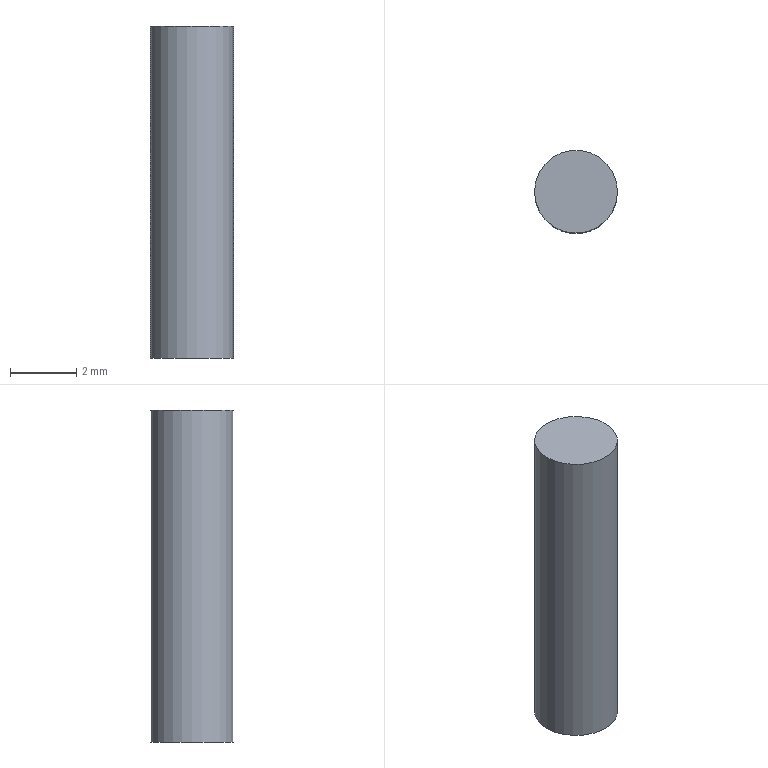Part | STEP file | 1 solid | 3 faces | box 2.5 x 2.5 x 10 mm | volume 49.087 mm3 | plane 2 | cylinder 1 | commonest cylinder face diameters 2.5 x1
STEP:
#1=CARTESIAN_POINT('',(0.,0.,0.));
#2=DIRECTION('',(0.,0.,1.));
#3=DIRECTION('',(1.,0.,0.));
#4=AXIS2_PLACEMENT_3D('',#1,#2,#3);
#5=CARTESIAN_POINT('',(1.25,0.,10.));
#6=VERTEX_POINT('',#5);
#7=CARTESIAN_POINT('',(0.,0.,10.));
#8=DIRECTION('',(0.,0.,-1.));
#9=DIRECTION('',(1.,0.,0.));
#10=AXIS2_PLACEMENT_3D('',#7,#8,#9);
#11=CIRCLE('',#10,1.25);
#12=CARTESIAN_POINT('',(0.,0.,0.));
#13=DIRECTION('',(0.,0.,1.));
#14=DIRECTION('',(1.,0.,0.));
#15=AXIS2_PLACEMENT_3D('',#12,#13,#14);
#16=CYLINDRICAL_SURFACE('',#15,1.25);
#17=CARTESIAN_POINT('',(6.283,10.));
#18=DIRECTION('',(-1.,0.));
#19=VECTOR('',#18,1.);
#20=LINE('',#17,#19);
#21=(GEOMETRIC_REPRESENTATION_CONTEXT(2)PARAMETRIC_REPRESENTATION_CONTEXT()REPRESENTATION_CONTEXT('',''));
#22=DEFINITIONAL_REPRESENTATION('',(#20),#21);
#23=PCURVE('',#16,#22);
#24=CARTESIAN_POINT('',(0.,0.,10.));
#25=DIRECTION('',(0.,0.,1.));
#26=DIRECTION('',(1.,0.,0.));
#27=AXIS2_PLACEMENT_3D('',#24,#25,#26);
#28=PLANE('',#27);
#29=CARTESIAN_POINT('',(1.25,0.));
#30=CARTESIAN_POINT('',(1.25,-2.165));
#31=CARTESIAN_POINT('',(-0.625,-1.083));
#32=CARTESIAN_POINT('',(-2.5,0.));
#33=CARTESIAN_POINT('',(-0.625,1.083));
#34=CARTESIAN_POINT('',(1.25,2.165));
#35=CARTESIAN_POINT('',(1.25,0.));
#36=(BOUNDED_CURVE()B_SPLINE_CURVE(2,(#29,#30,#31,#32,#33,#34,#35),.UNSPECIFIED.,.T.,.F.)B_SPLINE_CURVE_WITH_KNOTS((1,2,2,2,2,1),(-2.094,0.,2.094,4.189,6.283,8.378),.UNSPECIFIED.)CURVE()GEOMETRIC_REPRESENTATION_ITEM()RATIONAL_B_SPLINE_CURVE((1.,0.5,1.,0.5,1.,0.5,1.))REPRESENTATION_ITEM(''));
#37=(GEOMETRIC_REPRESENTATION_CONTEXT(2)PARAMETRIC_REPRESENTATION_CONTEXT()REPRESENTATION_CONTEXT('',''));
#38=DEFINITIONAL_REPRESENTATION('',(#36),#37);
#39=PCURVE('',#28,#38);
#40=SURFACE_CURVE('',#11,(#23,#39),.PCURVE_S1.);
#41=EDGE_CURVE('',#6,#6,#40,.T.);
#42=ORIENTED_EDGE('',*,*,#41,.T.);
#43=CARTESIAN_POINT('',(1.25,0.,0.));
#44=VERTEX_POINT('',#43);
#45=CARTESIAN_POINT('',(1.25,0.,0.));
#46=CARTESIAN_POINT('',(1.25,0.,10.));
#47=B_SPLINE_CURVE_WITH_KNOTS('',1,(#45,#46),.UNSPECIFIED.,.F.,.F.,(2,2),(0.,10.),.PIECEWISE_BEZIER_KNOTS.);
#48=CARTESIAN_POINT('',(0.,0.));
#49=DIRECTION('',(0.,1.));
#50=VECTOR('',#49,1.);
#51=LINE('',#48,#50);
#52=(GEOMETRIC_REPRESENTATION_CONTEXT(2)PARAMETRIC_REPRESENTATION_CONTEXT()REPRESENTATION_CONTEXT('',''));
#53=DEFINITIONAL_REPRESENTATION('',(#51),#52);
#54=PCURVE('',#16,#53);
#55=CARTESIAN_POINT('',(6.283,0.));
#56=DIRECTION('',(0.,1.));
#57=VECTOR('',#56,1.);
#58=LINE('',#55,#57);
#59=(GEOMETRIC_REPRESENTATION_CONTEXT(2)PARAMETRIC_REPRESENTATION_CONTEXT()REPRESENTATION_CONTEXT('',''));
#60=DEFINITIONAL_REPRESENTATION('',(#58),#59);
#61=PCURVE('',#16,#60);
#62=SEAM_CURVE('',#47,(#54,#61),.PCURVE_S1.);
#63=EDGE_CURVE('',#44,#6,#62,.T.);
#64=ORIENTED_EDGE('',*,*,#63,.F.);
#65=CARTESIAN_POINT('',(0.,0.,0.));
#66=DIRECTION('',(0.,0.,1.));
#67=DIRECTION('',(1.,0.,0.));
#68=AXIS2_PLACEMENT_3D('',#65,#66,#67);
#69=CIRCLE('',#68,1.25);
#70=CARTESIAN_POINT('',(0.,0.));
#71=DIRECTION('',(1.,0.));
#72=VECTOR('',#71,1.);
#73=LINE('',#70,#72);
#74=(GEOMETRIC_REPRESENTATION_CONTEXT(2)PARAMETRIC_REPRESENTATION_CONTEXT()REPRESENTATION_CONTEXT('',''));
#75=DEFINITIONAL_REPRESENTATION('',(#73),#74);
#76=PCURVE('',#16,#75);
#77=CARTESIAN_POINT('',(0.,0.,0.));
#78=DIRECTION('',(0.,0.,1.));
#79=DIRECTION('',(1.,0.,0.));
#80=AXIS2_PLACEMENT_3D('',#77,#78,#79);
#81=PLANE('',#80);
#82=CARTESIAN_POINT('',(0.,0.));
#83=DIRECTION('',(1.,0.));
#84=AXIS2_PLACEMENT_2D('',#82,#83);
#85=CIRCLE('',#84,1.25);
#86=(GEOMETRIC_REPRESENTATION_CONTEXT(2)PARAMETRIC_REPRESENTATION_CONTEXT()REPRESENTATION_CONTEXT('',''));
#87=DEFINITIONAL_REPRESENTATION('',(#85),#86);
#88=PCURVE('',#81,#87);
#89=SURFACE_CURVE('',#69,(#76,#88),.PCURVE_S1.);
#90=EDGE_CURVE('',#44,#44,#89,.T.);
#91=ORIENTED_EDGE('',*,*,#90,.T.);
#92=ORIENTED_EDGE('',*,*,#63,.T.);
#93=EDGE_LOOP('',(#42,#64,#91,#92));
#94=FACE_BOUND('',#93,.T.);
#95=ADVANCED_FACE('',(#94),#16,.T.);
#96=ORIENTED_EDGE('',*,*,#41,.F.);
#97=EDGE_LOOP('',(#96));
#98=FACE_BOUND('',#97,.T.);
#99=ADVANCED_FACE('',(#98),#28,.T.);
#100=ORIENTED_EDGE('',*,*,#90,.F.);
#101=EDGE_LOOP('',(#100));
#102=FACE_BOUND('',#101,.T.);
#103=ADVANCED_FACE('',(#102),#81,.F.);
#104=CLOSED_SHELL('',(#95,#99,#103));
#105=MANIFOLD_SOLID_BREP('',#104);
#106=(LENGTH_UNIT()NAMED_UNIT(*)SI_UNIT(.MILLI.,.METRE.));
#107=UNCERTAINTY_MEASURE_WITH_UNIT(LENGTH_MEASURE(0.00001),#106,'','');
#108=(NAMED_UNIT(*)PLANE_ANGLE_UNIT()SI_UNIT($,.RADIAN.));
#109=(NAMED_UNIT(*)SI_UNIT($,.STERADIAN.)SOLID_ANGLE_UNIT());
#110=(GEOMETRIC_REPRESENTATION_CONTEXT(3)GLOBAL_UNCERTAINTY_ASSIGNED_CONTEXT((#107))GLOBAL_UNIT_ASSIGNED_CONTEXT((#106,#108,#109))REPRESENTATION_CONTEXT('',''));
#111=ADVANCED_BREP_SHAPE_REPRESENTATION('',(#4,#105),#110);